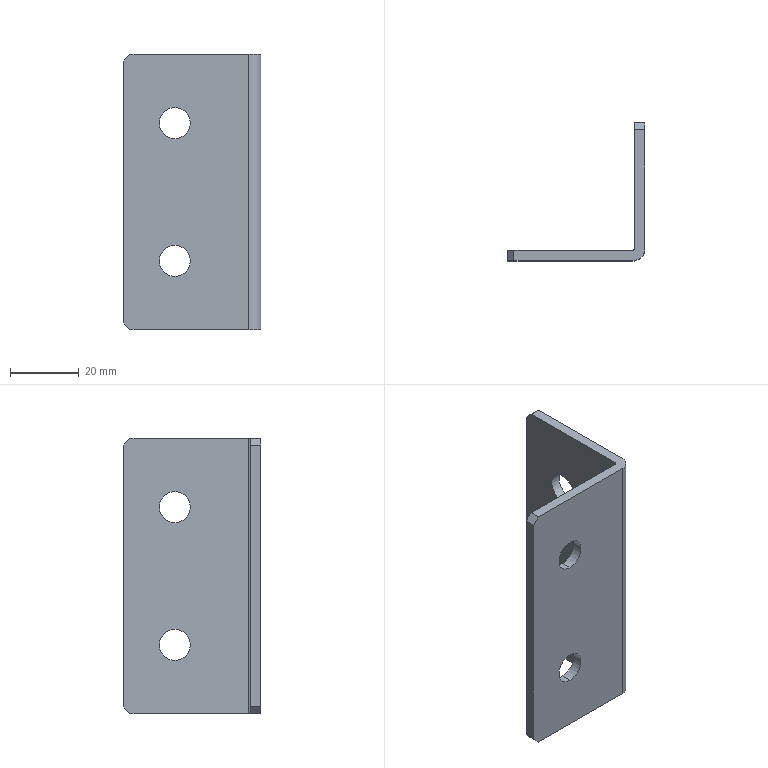Part | SolidWorks | features BaseBody 1 | 1 solid | 22 faces | box 40 x 40 x 80 mm | volume 17487 mm3 | plane 12 | cylinder 10 | commonest cylinder face diameters 9 x8 1 x1 7 x1
STEP:
#1=CARTESIAN_POINT('',(-25.,0.,55.5));
#2=VERTEX_POINT('',#1);
#3=CARTESIAN_POINT('',(-25.,0.,64.5));
#4=VERTEX_POINT('',#3);
#5=CARTESIAN_POINT('',(-25.,0.,60.));
#6=DIRECTION('',(0.,1.,0.));
#7=DIRECTION('',(0.,0.,1.));
#8=AXIS2_PLACEMENT_3D('',#5,#6,#7);
#9=CIRCLE('',#8,4.5);
#10=EDGE_CURVE('',#2,#4,#9,.T.);
#11=ORIENTED_EDGE('',*,*,#10,.F.);
#12=CARTESIAN_POINT('',(-25.,3.,55.5));
#13=VERTEX_POINT('',#12);
#14=CARTESIAN_POINT('',(-25.,3.,55.5));
#15=DIRECTION('',(0.,1.,0.));
#16=VECTOR('',#15,1000.);
#17=LINE('',#14,#16);
#18=EDGE_CURVE('',#2,#13,#17,.T.);
#19=ORIENTED_EDGE('',*,*,#18,.T.);
#20=CARTESIAN_POINT('',(-25.,3.,64.5));
#21=VERTEX_POINT('',#20);
#22=CARTESIAN_POINT('',(-25.,3.,60.));
#23=DIRECTION('',(0.,-1.,0.));
#24=DIRECTION('',(0.,0.,1.));
#25=AXIS2_PLACEMENT_3D('',#22,#23,#24);
#26=CIRCLE('',#25,4.5);
#27=EDGE_CURVE('',#21,#13,#26,.T.);
#28=ORIENTED_EDGE('',*,*,#27,.F.);
#29=CARTESIAN_POINT('',(-25.,3.,64.5));
#30=DIRECTION('',(0.,1.,0.));
#31=VECTOR('',#30,1000.);
#32=LINE('',#29,#31);
#33=EDGE_CURVE('',#4,#21,#32,.T.);
#34=ORIENTED_EDGE('',*,*,#33,.F.);
#35=EDGE_LOOP('',(#11,#19,#28,#34));
#36=FACE_OUTER_BOUND('',#35,.T.);
#37=CARTESIAN_POINT('',(-25.,3.,60.));
#38=DIRECTION('',(0.,1.,0.));
#39=DIRECTION('',(0.,0.,1.));
#40=AXIS2_PLACEMENT_3D('',#37,#38,#39);
#41=CYLINDRICAL_SURFACE('',#40,4.5);
#42=ADVANCED_FACE('',(#36),#41,.F.);
#43=CARTESIAN_POINT('',(-25.,0.,15.5));
#44=VERTEX_POINT('',#43);
#45=CARTESIAN_POINT('',(-25.,0.,24.5));
#46=VERTEX_POINT('',#45);
#47=CARTESIAN_POINT('',(-25.,0.,20.));
#48=DIRECTION('',(0.,1.,0.));
#49=DIRECTION('',(0.,0.,1.));
#50=AXIS2_PLACEMENT_3D('',#47,#48,#49);
#51=CIRCLE('',#50,4.5);
#52=EDGE_CURVE('',#44,#46,#51,.T.);
#53=ORIENTED_EDGE('',*,*,#52,.F.);
#54=CARTESIAN_POINT('',(-25.,3.,15.5));
#55=VERTEX_POINT('',#54);
#56=CARTESIAN_POINT('',(-25.,3.,15.5));
#57=DIRECTION('',(0.,1.,0.));
#58=VECTOR('',#57,1000.);
#59=LINE('',#56,#58);
#60=EDGE_CURVE('',#44,#55,#59,.T.);
#61=ORIENTED_EDGE('',*,*,#60,.T.);
#62=CARTESIAN_POINT('',(-25.,3.,24.5));
#63=VERTEX_POINT('',#62);
#64=CARTESIAN_POINT('',(-25.,3.,20.));
#65=DIRECTION('',(0.,-1.,0.));
#66=DIRECTION('',(0.,0.,1.));
#67=AXIS2_PLACEMENT_3D('',#64,#65,#66);
#68=CIRCLE('',#67,4.5);
#69=EDGE_CURVE('',#63,#55,#68,.T.);
#70=ORIENTED_EDGE('',*,*,#69,.F.);
#71=CARTESIAN_POINT('',(-25.,3.,24.5));
#72=DIRECTION('',(0.,1.,0.));
#73=VECTOR('',#72,1000.);
#74=LINE('',#71,#73);
#75=EDGE_CURVE('',#46,#63,#74,.T.);
#76=ORIENTED_EDGE('',*,*,#75,.F.);
#77=EDGE_LOOP('',(#53,#61,#70,#76));
#78=FACE_OUTER_BOUND('',#77,.T.);
#79=CARTESIAN_POINT('',(-25.,3.,20.));
#80=DIRECTION('',(0.,1.,0.));
#81=DIRECTION('',(0.,0.,1.));
#82=AXIS2_PLACEMENT_3D('',#79,#80,#81);
#83=CYLINDRICAL_SURFACE('',#82,4.5);
#84=ADVANCED_FACE('',(#78),#83,.F.);
#85=CARTESIAN_POINT('',(0.,25.,55.5));
#86=VERTEX_POINT('',#85);
#87=CARTESIAN_POINT('',(0.,25.,64.5));
#88=VERTEX_POINT('',#87);
#89=CARTESIAN_POINT('',(0.,25.,60.));
#90=DIRECTION('',(-1.,0.,0.));
#91=DIRECTION('',(0.,0.,1.));
#92=AXIS2_PLACEMENT_3D('',#89,#90,#91);
#93=CIRCLE('',#92,4.5);
#94=EDGE_CURVE('',#86,#88,#93,.T.);
#95=ORIENTED_EDGE('',*,*,#94,.F.);
#96=CARTESIAN_POINT('',(-3.,25.,55.5));
#97=VERTEX_POINT('',#96);
#98=CARTESIAN_POINT('',(-3.,25.,55.5));
#99=DIRECTION('',(-1.,0.,0.));
#100=VECTOR('',#99,1000.);
#101=LINE('',#98,#100);
#102=EDGE_CURVE('',#86,#97,#101,.T.);
#103=ORIENTED_EDGE('',*,*,#102,.T.);
#104=CARTESIAN_POINT('',(-3.,25.,64.5));
#105=VERTEX_POINT('',#104);
#106=CARTESIAN_POINT('',(-3.,25.,60.));
#107=DIRECTION('',(1.,0.,0.));
#108=DIRECTION('',(0.,0.,1.));
#109=AXIS2_PLACEMENT_3D('',#106,#107,#108);
#110=CIRCLE('',#109,4.5);
#111=EDGE_CURVE('',#105,#97,#110,.T.);
#112=ORIENTED_EDGE('',*,*,#111,.F.);
#113=CARTESIAN_POINT('',(-3.,25.,64.5));
#114=DIRECTION('',(-1.,0.,0.));
#115=VECTOR('',#114,1000.);
#116=LINE('',#113,#115);
#117=EDGE_CURVE('',#88,#105,#116,.T.);
#118=ORIENTED_EDGE('',*,*,#117,.F.);
#119=EDGE_LOOP('',(#95,#103,#112,#118));
#120=FACE_OUTER_BOUND('',#119,.T.);
#121=CARTESIAN_POINT('',(-3.,25.,60.));
#122=DIRECTION('',(-1.,0.,0.));
#123=DIRECTION('',(0.,0.,1.));
#124=AXIS2_PLACEMENT_3D('',#121,#122,#123);
#125=CYLINDRICAL_SURFACE('',#124,4.5);
#126=ADVANCED_FACE('',(#120),#125,.F.);
#127=CARTESIAN_POINT('',(0.,25.,15.5));
#128=VERTEX_POINT('',#127);
#129=CARTESIAN_POINT('',(0.,25.,24.5));
#130=VERTEX_POINT('',#129);
#131=CARTESIAN_POINT('',(0.,25.,20.));
#132=DIRECTION('',(-1.,0.,0.));
#133=DIRECTION('',(0.,0.,1.));
#134=AXIS2_PLACEMENT_3D('',#131,#132,#133);
#135=CIRCLE('',#134,4.5);
#136=EDGE_CURVE('',#128,#130,#135,.T.);
#137=ORIENTED_EDGE('',*,*,#136,.F.);
#138=CARTESIAN_POINT('',(-3.,25.,15.5));
#139=VERTEX_POINT('',#138);
#140=CARTESIAN_POINT('',(-3.,25.,15.5));
#141=DIRECTION('',(-1.,0.,0.));
#142=VECTOR('',#141,1000.);
#143=LINE('',#140,#142);
#144=EDGE_CURVE('',#128,#139,#143,.T.);
#145=ORIENTED_EDGE('',*,*,#144,.T.);
#146=CARTESIAN_POINT('',(-3.,25.,24.5));
#147=VERTEX_POINT('',#146);
#148=CARTESIAN_POINT('',(-3.,25.,20.));
#149=DIRECTION('',(1.,0.,0.));
#150=DIRECTION('',(0.,0.,1.));
#151=AXIS2_PLACEMENT_3D('',#148,#149,#150);
#152=CIRCLE('',#151,4.5);
#153=EDGE_CURVE('',#147,#139,#152,.T.);
#154=ORIENTED_EDGE('',*,*,#153,.F.);
#155=CARTESIAN_POINT('',(-3.,25.,24.5));
#156=DIRECTION('',(-1.,0.,0.));
#157=VECTOR('',#156,1000.);
#158=LINE('',#155,#157);
#159=EDGE_CURVE('',#130,#147,#158,.T.);
#160=ORIENTED_EDGE('',*,*,#159,.F.);
#161=EDGE_LOOP('',(#137,#145,#154,#160));
#162=FACE_OUTER_BOUND('',#161,.T.);
#163=CARTESIAN_POINT('',(-3.,25.,20.));
#164=DIRECTION('',(-1.,0.,0.));
#165=DIRECTION('',(0.,0.,1.));
#166=AXIS2_PLACEMENT_3D('',#163,#164,#165);
#167=CYLINDRICAL_SURFACE('',#166,4.5);
#168=ADVANCED_FACE('',(#162),#167,.F.);
#169=CARTESIAN_POINT('',(-3.5,0.,80.));
#170=VERTEX_POINT('',#169);
#171=CARTESIAN_POINT('',(-38.,0.,80.));
#172=VERTEX_POINT('',#171);
#173=CARTESIAN_POINT('',(0.,0.,80.));
#174=DIRECTION('',(-1.,0.,0.));
#175=VECTOR('',#174,1000.);
#176=LINE('',#173,#175);
#177=EDGE_CURVE('',#170,#172,#176,.T.);
#178=ORIENTED_EDGE('',*,*,#177,.T.);
#179=CARTESIAN_POINT('',(-40.,0.,78.));
#180=VERTEX_POINT('',#179);
#181=CARTESIAN_POINT('',(-38.,0.,80.));
#182=DIRECTION('',(-0.7071,0.,-0.7071));
#183=VECTOR('',#182,1000.);
#184=LINE('',#181,#183);
#185=EDGE_CURVE('',#172,#180,#184,.T.);
#186=ORIENTED_EDGE('',*,*,#185,.T.);
#187=CARTESIAN_POINT('',(-40.,0.,2.));
#188=VERTEX_POINT('',#187);
#189=CARTESIAN_POINT('',(-40.,0.,80.));
#190=DIRECTION('',(0.,0.,-1.));
#191=VECTOR('',#190,1000.);
#192=LINE('',#189,#191);
#193=EDGE_CURVE('',#180,#188,#192,.T.);
#194=ORIENTED_EDGE('',*,*,#193,.T.);
#195=CARTESIAN_POINT('',(-38.,0.,0.));
#196=VERTEX_POINT('',#195);
#197=CARTESIAN_POINT('',(-40.,0.,2.));
#198=DIRECTION('',(0.7071,0.,-0.7071));
#199=VECTOR('',#198,1000.);
#200=LINE('',#197,#199);
#201=EDGE_CURVE('',#188,#196,#200,.T.);
#202=ORIENTED_EDGE('',*,*,#201,.T.);
#203=CARTESIAN_POINT('',(-3.5,0.,0.));
#204=VERTEX_POINT('',#203);
#205=CARTESIAN_POINT('',(0.,0.,0.));
#206=DIRECTION('',(1.,0.,0.));
#207=VECTOR('',#206,1000.);
#208=LINE('',#205,#207);
#209=EDGE_CURVE('',#196,#204,#208,.T.);
#210=ORIENTED_EDGE('',*,*,#209,.T.);
#211=CARTESIAN_POINT('',(-3.5,0.,80.));
#212=DIRECTION('',(0.,0.,1.));
#213=VECTOR('',#212,1000.);
#214=LINE('',#211,#213);
#215=EDGE_CURVE('',#204,#170,#214,.T.);
#216=ORIENTED_EDGE('',*,*,#215,.T.);
#217=EDGE_LOOP('',(#178,#186,#194,#202,#210,#216));
#218=FACE_OUTER_BOUND('',#217,.T.);
#219=CARTESIAN_POINT('',(-25.,0.,60.));
#220=DIRECTION('',(0.,1.,0.));
#221=DIRECTION('',(0.,0.,1.));
#222=AXIS2_PLACEMENT_3D('',#219,#220,#221);
#223=CIRCLE('',#222,4.5);
#224=EDGE_CURVE('',#4,#2,#223,.T.);
#225=ORIENTED_EDGE('',*,*,#224,.T.);
#226=ORIENTED_EDGE('',*,*,#10,.T.);
#227=EDGE_LOOP('',(#225,#226));
#228=FACE_BOUND('',#227,.T.);
#229=CARTESIAN_POINT('',(-25.,0.,20.));
#230=DIRECTION('',(0.,1.,0.));
#231=DIRECTION('',(0.,0.,1.));
#232=AXIS2_PLACEMENT_3D('',#229,#230,#231);
#233=CIRCLE('',#232,4.5);
#234=EDGE_CURVE('',#46,#44,#233,.T.);
#235=ORIENTED_EDGE('',*,*,#234,.T.);
#236=ORIENTED_EDGE('',*,*,#52,.T.);
#237=EDGE_LOOP('',(#235,#236));
#238=FACE_BOUND('',#237,.T.);
#239=CARTESIAN_POINT('',(0.,0.,80.));
#240=DIRECTION('',(0.,-1.,0.));
#241=DIRECTION('',(0.,0.,-1.));
#242=AXIS2_PLACEMENT_3D('',#239,#240,#241);
#243=PLANE('',#242);
#244=ADVANCED_FACE('',(#218,#228,#238),#243,.T.);
#245=CARTESIAN_POINT('',(-38.,3.,80.));
#246=VERTEX_POINT('',#245);
#247=CARTESIAN_POINT('',(-38.,0.,80.));
#248=DIRECTION('',(0.,-1.,0.));
#249=VECTOR('',#248,1000.);
#250=LINE('',#247,#249);
#251=EDGE_CURVE('',#246,#172,#250,.T.);
#252=ORIENTED_EDGE('',*,*,#251,.F.);
#253=CARTESIAN_POINT('',(-40.,3.,78.));
#254=VERTEX_POINT('',#253);
#255=CARTESIAN_POINT('',(-40.,3.,78.));
#256=DIRECTION('',(0.7071,0.,0.7071));
#257=VECTOR('',#256,1000.);
#258=LINE('',#255,#257);
#259=EDGE_CURVE('',#254,#246,#258,.T.);
#260=ORIENTED_EDGE('',*,*,#259,.F.);
#261=CARTESIAN_POINT('',(-40.,0.,78.));
#262=DIRECTION('',(0.,1.,0.));
#263=VECTOR('',#262,1000.);
#264=LINE('',#261,#263);
#265=EDGE_CURVE('',#180,#254,#264,.T.);
#266=ORIENTED_EDGE('',*,*,#265,.F.);
#267=ORIENTED_EDGE('',*,*,#185,.F.);
#268=EDGE_LOOP('',(#252,#260,#266,#267));
#269=FACE_OUTER_BOUND('',#268,.T.);
#270=CARTESIAN_POINT('',(-40.,0.,78.));
#271=DIRECTION('',(0.7071,0.,-0.7071));
#272=DIRECTION('',(-0.7071,0.,-0.7071));
#273=AXIS2_PLACEMENT_3D('',#270,#271,#272);
#274=PLANE('',#273);
#275=ADVANCED_FACE('',(#269),#274,.F.);
#276=ORIENTED_EDGE('',*,*,#177,.F.);
#277=CARTESIAN_POINT('',(0.,3.5,80.));
#278=VERTEX_POINT('',#277);
#279=CARTESIAN_POINT('',(-3.5,3.5,80.));
#280=DIRECTION('',(0.,0.,-1.));
#281=DIRECTION('',(-1.,0.,0.));
#282=AXIS2_PLACEMENT_3D('',#279,#280,#281);
#283=CIRCLE('',#282,3.5);
#284=EDGE_CURVE('',#278,#170,#283,.T.);
#285=ORIENTED_EDGE('',*,*,#284,.F.);
#286=CARTESIAN_POINT('',(0.,38.,80.));
#287=VERTEX_POINT('',#286);
#288=CARTESIAN_POINT('',(0.,40.,80.));
#289=DIRECTION('',(0.,-1.,0.));
#290=VECTOR('',#289,1000.);
#291=LINE('',#288,#290);
#292=EDGE_CURVE('',#287,#278,#291,.T.);
#293=ORIENTED_EDGE('',*,*,#292,.F.);
#294=CARTESIAN_POINT('',(-3.,38.,80.));
#295=VERTEX_POINT('',#294);
#296=CARTESIAN_POINT('',(-3.5,38.,80.));
#297=DIRECTION('',(-1.,0.,0.));
#298=VECTOR('',#297,1000.);
#299=LINE('',#296,#298);
#300=EDGE_CURVE('',#287,#295,#299,.T.);
#301=ORIENTED_EDGE('',*,*,#300,.T.);
#302=CARTESIAN_POINT('',(-3.,3.5,80.));
#303=VERTEX_POINT('',#302);
#304=CARTESIAN_POINT('',(-3.,3.5,80.));
#305=DIRECTION('',(0.,-1.,0.));
#306=VECTOR('',#305,1000.);
#307=LINE('',#304,#306);
#308=EDGE_CURVE('',#295,#303,#307,.T.);
#309=ORIENTED_EDGE('',*,*,#308,.T.);
#310=CARTESIAN_POINT('',(-3.5,3.,80.));
#311=VERTEX_POINT('',#310);
#312=CARTESIAN_POINT('',(-3.5,3.5,80.));
#313=DIRECTION('',(0.,0.,-1.));
#314=DIRECTION('',(-1.,0.,0.));
#315=AXIS2_PLACEMENT_3D('',#312,#313,#314);
#316=CIRCLE('',#315,0.5);
#317=EDGE_CURVE('',#303,#311,#316,.T.);
#318=ORIENTED_EDGE('',*,*,#317,.T.);
#319=CARTESIAN_POINT('',(-3.,3.,80.));
#320=DIRECTION('',(-1.,0.,0.));
#321=VECTOR('',#320,1000.);
#322=LINE('',#319,#321);
#323=EDGE_CURVE('',#311,#246,#322,.T.);
#324=ORIENTED_EDGE('',*,*,#323,.T.);
#325=ORIENTED_EDGE('',*,*,#251,.T.);
#326=EDGE_LOOP('',(#276,#285,#293,#301,#309,#318,#324,#325));
#327=FACE_OUTER_BOUND('',#326,.T.);
#328=CARTESIAN_POINT('',(-3.,3.5,80.));
#329=DIRECTION('',(0.,0.,1.));
#330=DIRECTION('',(1.,0.,0.));
#331=AXIS2_PLACEMENT_3D('',#328,#329,#330);
#332=PLANE('',#331);
#333=ADVANCED_FACE('',(#327),#332,.T.);
#334=ORIENTED_EDGE('',*,*,#284,.T.);
#335=ORIENTED_EDGE('',*,*,#215,.F.);
#336=CARTESIAN_POINT('',(0.,3.5,0.));
#337=VERTEX_POINT('',#336);
#338=CARTESIAN_POINT('',(-3.5,3.5,0.));
#339=DIRECTION('',(0.,0.,1.));
#340=DIRECTION('',(-1.,0.,0.));
#341=AXIS2_PLACEMENT_3D('',#338,#339,#340);
#342=CIRCLE('',#341,3.5);
#343=EDGE_CURVE('',#204,#337,#342,.T.);
#344=ORIENTED_EDGE('',*,*,#343,.T.);
#345=CARTESIAN_POINT('',(0.,3.5,80.));
#346=DIRECTION('',(0.,0.,1.));
#347=VECTOR('',#346,1000.);
#348=LINE('',#345,#347);
#349=EDGE_CURVE('',#337,#278,#348,.T.);
#350=ORIENTED_EDGE('',*,*,#349,.T.);
#351=EDGE_LOOP('',(#334,#335,#344,#350));
#352=FACE_OUTER_BOUND('',#351,.T.);
#353=CARTESIAN_POINT('',(-3.5,3.5,80.));
#354=DIRECTION('',(0.,0.,-1.));
#355=DIRECTION('',(-1.,0.,0.));
#356=AXIS2_PLACEMENT_3D('',#353,#354,#355);
#357=CYLINDRICAL_SURFACE('',#356,3.5);
#358=ADVANCED_FACE('',(#352),#357,.T.);
#359=CARTESIAN_POINT('',(-38.,3.,0.));
#360=VERTEX_POINT('',#359);
#361=CARTESIAN_POINT('',(-38.,3.5,0.));
#362=DIRECTION('',(0.,-1.,0.));
#363=VECTOR('',#362,1000.);
#364=LINE('',#361,#363);
#365=EDGE_CURVE('',#360,#196,#364,.T.);
#366=ORIENTED_EDGE('',*,*,#365,.F.);
#367=CARTESIAN_POINT('',(-3.5,3.,0.));
#368=VERTEX_POINT('',#367);
#369=CARTESIAN_POINT('',(-3.5,3.,0.));
#370=DIRECTION('',(-1.,0.,0.));
#371=VECTOR('',#370,1000.);
#372=LINE('',#369,#371);
#373=EDGE_CURVE('',#368,#360,#372,.T.);
#374=ORIENTED_EDGE('',*,*,#373,.F.);
#375=CARTESIAN_POINT('',(-3.,3.5,0.));
#376=VERTEX_POINT('',#375);
#377=CARTESIAN_POINT('',(-3.5,3.5,0.));
#378=DIRECTION('',(0.,0.,1.));
#379=DIRECTION('',(-1.,0.,0.));
#380=AXIS2_PLACEMENT_3D('',#377,#378,#379);
#381=CIRCLE('',#380,0.5);
#382=EDGE_CURVE('',#368,#376,#381,.T.);
#383=ORIENTED_EDGE('',*,*,#382,.T.);
#384=CARTESIAN_POINT('',(-3.,38.,0.));
#385=VERTEX_POINT('',#384);
#386=CARTESIAN_POINT('',(-3.,3.,0.));
#387=DIRECTION('',(0.,1.,0.));
#388=VECTOR('',#387,1000.);
#389=LINE('',#386,#388);
#390=EDGE_CURVE('',#376,#385,#389,.T.);
#391=ORIENTED_EDGE('',*,*,#390,.T.);
#392=CARTESIAN_POINT('',(0.,38.,0.));
#393=VERTEX_POINT('',#392);
#394=CARTESIAN_POINT('',(-3.5,38.,0.));
#395=DIRECTION('',(1.,0.,0.));
#396=VECTOR('',#395,1000.);
#397=LINE('',#394,#396);
#398=EDGE_CURVE('',#385,#393,#397,.T.);
#399=ORIENTED_EDGE('',*,*,#398,.T.);
#400=CARTESIAN_POINT('',(0.,40.,0.));
#401=DIRECTION('',(0.,1.,0.));
#402=VECTOR('',#401,1000.);
#403=LINE('',#400,#402);
#404=EDGE_CURVE('',#337,#393,#403,.T.);
#405=ORIENTED_EDGE('',*,*,#404,.F.);
#406=ORIENTED_EDGE('',*,*,#343,.F.);
#407=ORIENTED_EDGE('',*,*,#209,.F.);
#408=EDGE_LOOP('',(#366,#374,#383,#391,#399,#405,#406,#407));
#409=FACE_OUTER_BOUND('',#408,.T.);
#410=CARTESIAN_POINT('',(-3.5,3.5,0.));
#411=DIRECTION('',(0.,0.,1.));
#412=DIRECTION('',(1.,0.,0.));
#413=AXIS2_PLACEMENT_3D('',#410,#411,#412);
#414=PLANE('',#413);
#415=ADVANCED_FACE('',(#409),#414,.F.);
#416=CARTESIAN_POINT('',(-40.,3.,2.));
#417=VERTEX_POINT('',#416);
#418=CARTESIAN_POINT('',(-38.,3.,0.));
#419=DIRECTION('',(0.7071,0.,-0.7071));
#420=VECTOR('',#419,1000.);
#421=LINE('',#418,#420);
#422=EDGE_CURVE('',#417,#360,#421,.T.);
#423=ORIENTED_EDGE('',*,*,#422,.T.);
#424=ORIENTED_EDGE('',*,*,#365,.T.);
#425=ORIENTED_EDGE('',*,*,#201,.F.);
#426=CARTESIAN_POINT('',(-40.,3.5,2.));
#427=DIRECTION('',(0.,1.,0.));
#428=VECTOR('',#427,1000.);
#429=LINE('',#426,#428);
#430=EDGE_CURVE('',#188,#417,#429,.T.);
#431=ORIENTED_EDGE('',*,*,#430,.T.);
#432=EDGE_LOOP('',(#423,#424,#425,#431));
#433=FACE_OUTER_BOUND('',#432,.T.);
#434=CARTESIAN_POINT('',(-38.,3.5,0.));
#435=DIRECTION('',(-0.7071,0.,-0.7071));
#436=DIRECTION('',(-0.7071,0.,0.7071));
#437=AXIS2_PLACEMENT_3D('',#434,#435,#436);
#438=PLANE('',#437);
#439=ADVANCED_FACE('',(#433),#438,.T.);
#440=ORIENTED_EDGE('',*,*,#193,.F.);
#441=ORIENTED_EDGE('',*,*,#265,.T.);
#442=CARTESIAN_POINT('',(-40.,3.,80.));
#443=DIRECTION('',(0.,0.,-1.));
#444=VECTOR('',#443,1000.);
#445=LINE('',#442,#444);
#446=EDGE_CURVE('',#254,#417,#445,.T.);
#447=ORIENTED_EDGE('',*,*,#446,.T.);
#448=ORIENTED_EDGE('',*,*,#430,.F.);
#449=EDGE_LOOP('',(#440,#441,#447,#448));
#450=FACE_OUTER_BOUND('',#449,.T.);
#451=CARTESIAN_POINT('',(-40.,0.,80.));
#452=DIRECTION('',(-1.,0.,0.));
#453=DIRECTION('',(0.,0.,1.));
#454=AXIS2_PLACEMENT_3D('',#451,#452,#453);
#455=PLANE('',#454);
#456=ADVANCED_FACE('',(#450),#455,.T.);
#457=ORIENTED_EDGE('',*,*,#18,.F.);
#458=ORIENTED_EDGE('',*,*,#224,.F.);
#459=ORIENTED_EDGE('',*,*,#33,.T.);
#460=CARTESIAN_POINT('',(-25.,3.,60.));
#461=DIRECTION('',(0.,-1.,0.));
#462=DIRECTION('',(0.,0.,1.));
#463=AXIS2_PLACEMENT_3D('',#460,#461,#462);
#464=CIRCLE('',#463,4.5);
#465=EDGE_CURVE('',#13,#21,#464,.T.);
#466=ORIENTED_EDGE('',*,*,#465,.F.);
#467=EDGE_LOOP('',(#457,#458,#459,#466));
#468=FACE_OUTER_BOUND('',#467,.T.);
#469=CARTESIAN_POINT('',(-25.,3.,60.));
#470=DIRECTION('',(0.,1.,0.));
#471=DIRECTION('',(0.,0.,1.));
#472=AXIS2_PLACEMENT_3D('',#469,#470,#471);
#473=CYLINDRICAL_SURFACE('',#472,4.5);
#474=ADVANCED_FACE('',(#468),#473,.F.);
#475=ORIENTED_EDGE('',*,*,#60,.F.);
#476=ORIENTED_EDGE('',*,*,#234,.F.);
#477=ORIENTED_EDGE('',*,*,#75,.T.);
#478=CARTESIAN_POINT('',(-25.,3.,20.));
#479=DIRECTION('',(0.,-1.,0.));
#480=DIRECTION('',(0.,0.,1.));
#481=AXIS2_PLACEMENT_3D('',#478,#479,#480);
#482=CIRCLE('',#481,4.5);
#483=EDGE_CURVE('',#55,#63,#482,.T.);
#484=ORIENTED_EDGE('',*,*,#483,.F.);
#485=EDGE_LOOP('',(#475,#476,#477,#484));
#486=FACE_OUTER_BOUND('',#485,.T.);
#487=CARTESIAN_POINT('',(-25.,3.,20.));
#488=DIRECTION('',(0.,1.,0.));
#489=DIRECTION('',(0.,0.,1.));
#490=AXIS2_PLACEMENT_3D('',#487,#488,#489);
#491=CYLINDRICAL_SURFACE('',#490,4.5);
#492=ADVANCED_FACE('',(#486),#491,.F.);
#493=ORIENTED_EDGE('',*,*,#422,.F.);
#494=ORIENTED_EDGE('',*,*,#446,.F.);
#495=ORIENTED_EDGE('',*,*,#259,.T.);
#496=ORIENTED_EDGE('',*,*,#323,.F.);
#497=CARTESIAN_POINT('',(-3.5,3.,80.));
#498=DIRECTION('',(0.,0.,1.));
#499=VECTOR('',#498,1000.);
#500=LINE('',#497,#499);
#501=EDGE_CURVE('',#368,#311,#500,.T.);
#502=ORIENTED_EDGE('',*,*,#501,.F.);
#503=ORIENTED_EDGE('',*,*,#373,.T.);
#504=EDGE_LOOP('',(#493,#494,#495,#496,#502,#503));
#505=FACE_OUTER_BOUND('',#504,.T.);
#506=ORIENTED_EDGE('',*,*,#27,.T.);
#507=ORIENTED_EDGE('',*,*,#465,.T.);
#508=EDGE_LOOP('',(#506,#507));
#509=FACE_BOUND('',#508,.T.);
#510=ORIENTED_EDGE('',*,*,#69,.T.);
#511=ORIENTED_EDGE('',*,*,#483,.T.);
#512=EDGE_LOOP('',(#510,#511));
#513=FACE_BOUND('',#512,.T.);
#514=CARTESIAN_POINT('',(0.,3.,80.));
#515=DIRECTION('',(0.,-1.,0.));
#516=DIRECTION('',(0.,0.,-1.));
#517=AXIS2_PLACEMENT_3D('',#514,#515,#516);
#518=PLANE('',#517);
#519=ADVANCED_FACE('',(#505,#509,#513),#518,.F.);
#520=ORIENTED_EDGE('',*,*,#404,.T.);
#521=CARTESIAN_POINT('',(0.,40.,2.));
#522=VERTEX_POINT('',#521);
#523=CARTESIAN_POINT('',(0.,38.,0.));
#524=DIRECTION('',(0.,0.7071,0.7071));
#525=VECTOR('',#524,1000.);
#526=LINE('',#523,#525);
#527=EDGE_CURVE('',#393,#522,#526,.T.);
#528=ORIENTED_EDGE('',*,*,#527,.T.);
#529=CARTESIAN_POINT('',(0.,40.,78.));
#530=VERTEX_POINT('',#529);
#531=CARTESIAN_POINT('',(0.,40.,80.));
#532=DIRECTION('',(0.,0.,1.));
#533=VECTOR('',#532,1000.);
#534=LINE('',#531,#533);
#535=EDGE_CURVE('',#522,#530,#534,.T.);
#536=ORIENTED_EDGE('',*,*,#535,.T.);
#537=CARTESIAN_POINT('',(0.,40.,78.));
#538=DIRECTION('',(0.,-0.7071,0.7071));
#539=VECTOR('',#538,1000.);
#540=LINE('',#537,#539);
#541=EDGE_CURVE('',#530,#287,#540,.T.);
#542=ORIENTED_EDGE('',*,*,#541,.T.);
#543=ORIENTED_EDGE('',*,*,#292,.T.);
#544=ORIENTED_EDGE('',*,*,#349,.F.);
#545=EDGE_LOOP('',(#520,#528,#536,#542,#543,#544));
#546=FACE_OUTER_BOUND('',#545,.T.);
#547=CARTESIAN_POINT('',(0.,25.,60.));
#548=DIRECTION('',(-1.,0.,0.));
#549=DIRECTION('',(0.,0.,1.));
#550=AXIS2_PLACEMENT_3D('',#547,#548,#549);
#551=CIRCLE('',#550,4.5);
#552=EDGE_CURVE('',#88,#86,#551,.T.);
#553=ORIENTED_EDGE('',*,*,#552,.T.);
#554=ORIENTED_EDGE('',*,*,#94,.T.);
#555=EDGE_LOOP('',(#553,#554));
#556=FACE_BOUND('',#555,.T.);
#557=CARTESIAN_POINT('',(0.,25.,20.));
#558=DIRECTION('',(-1.,0.,0.));
#559=DIRECTION('',(0.,0.,1.));
#560=AXIS2_PLACEMENT_3D('',#557,#558,#559);
#561=CIRCLE('',#560,4.5);
#562=EDGE_CURVE('',#130,#128,#561,.T.);
#563=ORIENTED_EDGE('',*,*,#562,.T.);
#564=ORIENTED_EDGE('',*,*,#136,.T.);
#565=EDGE_LOOP('',(#563,#564));
#566=FACE_BOUND('',#565,.T.);
#567=CARTESIAN_POINT('',(0.,40.,80.));
#568=DIRECTION('',(1.,0.,0.));
#569=DIRECTION('',(0.,1.,0.));
#570=AXIS2_PLACEMENT_3D('',#567,#568,#569);
#571=PLANE('',#570);
#572=ADVANCED_FACE('',(#546,#556,#566),#571,.T.);
#573=ORIENTED_EDGE('',*,*,#501,.T.);
#574=ORIENTED_EDGE('',*,*,#317,.F.);
#575=CARTESIAN_POINT('',(-3.,3.5,80.));
#576=DIRECTION('',(0.,0.,1.));
#577=VECTOR('',#576,1000.);
#578=LINE('',#575,#577);
#579=EDGE_CURVE('',#376,#303,#578,.T.);
#580=ORIENTED_EDGE('',*,*,#579,.F.);
#581=ORIENTED_EDGE('',*,*,#382,.F.);
#582=EDGE_LOOP('',(#573,#574,#580,#581));
#583=FACE_OUTER_BOUND('',#582,.T.);
#584=CARTESIAN_POINT('',(-3.5,3.5,80.));
#585=DIRECTION('',(0.,0.,-1.));
#586=DIRECTION('',(-1.,0.,0.));
#587=AXIS2_PLACEMENT_3D('',#584,#585,#586);
#588=CYLINDRICAL_SURFACE('',#587,0.5);
#589=ADVANCED_FACE('',(#583),#588,.F.);
#590=CARTESIAN_POINT('',(-3.,40.,2.));
#591=VERTEX_POINT('',#590);
#592=CARTESIAN_POINT('',(-3.5,40.,2.));
#593=DIRECTION('',(-1.,0.,0.));
#594=VECTOR('',#593,1000.);
#595=LINE('',#592,#594);
#596=EDGE_CURVE('',#522,#591,#595,.T.);
#597=ORIENTED_EDGE('',*,*,#596,.F.);
#598=ORIENTED_EDGE('',*,*,#527,.F.);
#599=ORIENTED_EDGE('',*,*,#398,.F.);
#600=CARTESIAN_POINT('',(-3.,38.,0.));
#601=DIRECTION('',(0.,-0.7071,-0.7071));
#602=VECTOR('',#601,1000.);
#603=LINE('',#600,#602);
#604=EDGE_CURVE('',#591,#385,#603,.T.);
#605=ORIENTED_EDGE('',*,*,#604,.F.);
#606=EDGE_LOOP('',(#597,#598,#599,#605));
#607=FACE_OUTER_BOUND('',#606,.T.);
#608=CARTESIAN_POINT('',(-3.5,38.,0.));
#609=DIRECTION('',(0.,-0.7071,0.7071));
#610=DIRECTION('',(0.,-0.7071,-0.7071));
#611=AXIS2_PLACEMENT_3D('',#608,#609,#610);
#612=PLANE('',#611);
#613=ADVANCED_FACE('',(#607),#612,.F.);
#614=ORIENTED_EDGE('',*,*,#300,.F.);
#615=ORIENTED_EDGE('',*,*,#541,.F.);
#616=CARTESIAN_POINT('',(-3.,40.,78.));
#617=VERTEX_POINT('',#616);
#618=CARTESIAN_POINT('',(-3.,40.,78.));
#619=DIRECTION('',(1.,0.,0.));
#620=VECTOR('',#619,1000.);
#621=LINE('',#618,#620);
#622=EDGE_CURVE('',#617,#530,#621,.T.);
#623=ORIENTED_EDGE('',*,*,#622,.F.);
#624=CARTESIAN_POINT('',(-3.,40.,78.));
#625=DIRECTION('',(0.,0.7071,-0.7071));
#626=VECTOR('',#625,1000.);
#627=LINE('',#624,#626);
#628=EDGE_CURVE('',#295,#617,#627,.T.);
#629=ORIENTED_EDGE('',*,*,#628,.F.);
#630=EDGE_LOOP('',(#614,#615,#623,#629));
#631=FACE_OUTER_BOUND('',#630,.T.);
#632=CARTESIAN_POINT('',(-3.,40.,78.));
#633=DIRECTION('',(0.,-0.7071,-0.7071));
#634=DIRECTION('',(0.,0.7071,-0.7071));
#635=AXIS2_PLACEMENT_3D('',#632,#633,#634);
#636=PLANE('',#635);
#637=ADVANCED_FACE('',(#631),#636,.F.);
#638=ORIENTED_EDGE('',*,*,#535,.F.);
#639=ORIENTED_EDGE('',*,*,#596,.T.);
#640=CARTESIAN_POINT('',(-3.,40.,80.));
#641=DIRECTION('',(0.,0.,1.));
#642=VECTOR('',#641,1000.);
#643=LINE('',#640,#642);
#644=EDGE_CURVE('',#591,#617,#643,.T.);
#645=ORIENTED_EDGE('',*,*,#644,.T.);
#646=ORIENTED_EDGE('',*,*,#622,.T.);
#647=EDGE_LOOP('',(#638,#639,#645,#646));
#648=FACE_OUTER_BOUND('',#647,.T.);
#649=CARTESIAN_POINT('',(-3.,40.,80.));
#650=DIRECTION('',(0.,1.,0.));
#651=DIRECTION('',(0.,0.,1.));
#652=AXIS2_PLACEMENT_3D('',#649,#650,#651);
#653=PLANE('',#652);
#654=ADVANCED_FACE('',(#648),#653,.T.);
#655=ORIENTED_EDGE('',*,*,#102,.F.);
#656=ORIENTED_EDGE('',*,*,#552,.F.);
#657=ORIENTED_EDGE('',*,*,#117,.T.);
#658=CARTESIAN_POINT('',(-3.,25.,60.));
#659=DIRECTION('',(1.,0.,0.));
#660=DIRECTION('',(0.,0.,1.));
#661=AXIS2_PLACEMENT_3D('',#658,#659,#660);
#662=CIRCLE('',#661,4.5);
#663=EDGE_CURVE('',#97,#105,#662,.T.);
#664=ORIENTED_EDGE('',*,*,#663,.F.);
#665=EDGE_LOOP('',(#655,#656,#657,#664));
#666=FACE_OUTER_BOUND('',#665,.T.);
#667=CARTESIAN_POINT('',(-3.,25.,60.));
#668=DIRECTION('',(-1.,0.,0.));
#669=DIRECTION('',(0.,0.,1.));
#670=AXIS2_PLACEMENT_3D('',#667,#668,#669);
#671=CYLINDRICAL_SURFACE('',#670,4.5);
#672=ADVANCED_FACE('',(#666),#671,.F.);
#673=ORIENTED_EDGE('',*,*,#144,.F.);
#674=ORIENTED_EDGE('',*,*,#562,.F.);
#675=ORIENTED_EDGE('',*,*,#159,.T.);
#676=CARTESIAN_POINT('',(-3.,25.,20.));
#677=DIRECTION('',(1.,0.,0.));
#678=DIRECTION('',(0.,0.,1.));
#679=AXIS2_PLACEMENT_3D('',#676,#677,#678);
#680=CIRCLE('',#679,4.5);
#681=EDGE_CURVE('',#139,#147,#680,.T.);
#682=ORIENTED_EDGE('',*,*,#681,.F.);
#683=EDGE_LOOP('',(#673,#674,#675,#682));
#684=FACE_OUTER_BOUND('',#683,.T.);
#685=CARTESIAN_POINT('',(-3.,25.,20.));
#686=DIRECTION('',(-1.,0.,0.));
#687=DIRECTION('',(0.,0.,1.));
#688=AXIS2_PLACEMENT_3D('',#685,#686,#687);
#689=CYLINDRICAL_SURFACE('',#688,4.5);
#690=ADVANCED_FACE('',(#684),#689,.F.);
#691=ORIENTED_EDGE('',*,*,#628,.T.);
#692=ORIENTED_EDGE('',*,*,#644,.F.);
#693=ORIENTED_EDGE('',*,*,#604,.T.);
#694=ORIENTED_EDGE('',*,*,#390,.F.);
#695=ORIENTED_EDGE('',*,*,#579,.T.);
#696=ORIENTED_EDGE('',*,*,#308,.F.);
#697=EDGE_LOOP('',(#691,#692,#693,#694,#695,#696));
#698=FACE_OUTER_BOUND('',#697,.T.);
#699=ORIENTED_EDGE('',*,*,#111,.T.);
#700=ORIENTED_EDGE('',*,*,#663,.T.);
#701=EDGE_LOOP('',(#699,#700));
#702=FACE_BOUND('',#701,.T.);
#703=ORIENTED_EDGE('',*,*,#153,.T.);
#704=ORIENTED_EDGE('',*,*,#681,.T.);
#705=EDGE_LOOP('',(#703,#704));
#706=FACE_BOUND('',#705,.T.);
#707=CARTESIAN_POINT('',(-3.,40.,80.));
#708=DIRECTION('',(1.,0.,0.));
#709=DIRECTION('',(0.,1.,0.));
#710=AXIS2_PLACEMENT_3D('',#707,#708,#709);
#711=PLANE('',#710);
#712=ADVANCED_FACE('',(#698,#702,#706),#711,.F.);
#713=CLOSED_SHELL('',(#42,#84,#126,#168,#244,#275,#333,#358,#415,#439,#456,#474,#492,#519,#572,#589,#613,#637,#654,#672,#690,#712));
#714=MANIFOLD_SOLID_BREP('',#713);
#715=CARTESIAN_POINT('',(0.,0.,0.));
#716=DIRECTION('',(0.,0.,1.));
#717=DIRECTION('',(1.,0.,0.));
#718=AXIS2_PLACEMENT_3D('',#715,#716,#717);
#719=(LENGTH_UNIT()NAMED_UNIT(*)SI_UNIT(.MILLI.,.METRE.));
#720=UNCERTAINTY_MEASURE_WITH_UNIT(LENGTH_MEASURE(0.00001),#719,'','');
#721=(NAMED_UNIT(*)PLANE_ANGLE_UNIT()SI_UNIT($,.RADIAN.));
#722=(NAMED_UNIT(*)SI_UNIT($,.STERADIAN.)SOLID_ANGLE_UNIT());
#723=(GEOMETRIC_REPRESENTATION_CONTEXT(3)GLOBAL_UNCERTAINTY_ASSIGNED_CONTEXT((#720))GLOBAL_UNIT_ASSIGNED_CONTEXT((#719,#721,#722))REPRESENTATION_CONTEXT('',''));
#724=ADVANCED_BREP_SHAPE_REPRESENTATION('',(#714,#718),#723);